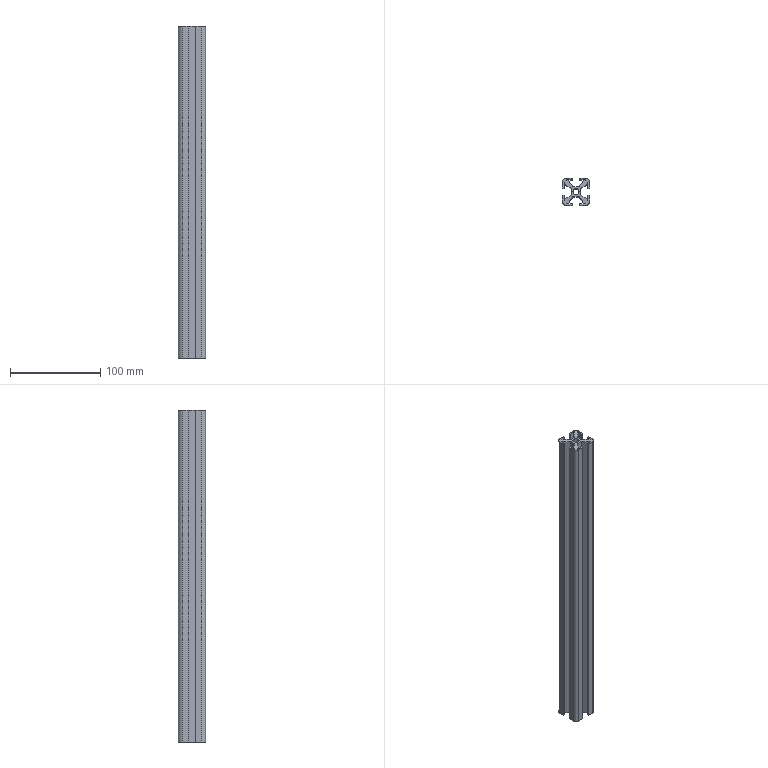Part | SolidWorks | features CirPattern 1, Extrusion 1, Fillet 1, ICE 1 | 1 solid | 60 faces | box 30 x 30 x 367 mm | volume 143787 mm3 | plane 54 | cylinder 6 | commonest cylinder face diameters 9 x4 6.8 x2